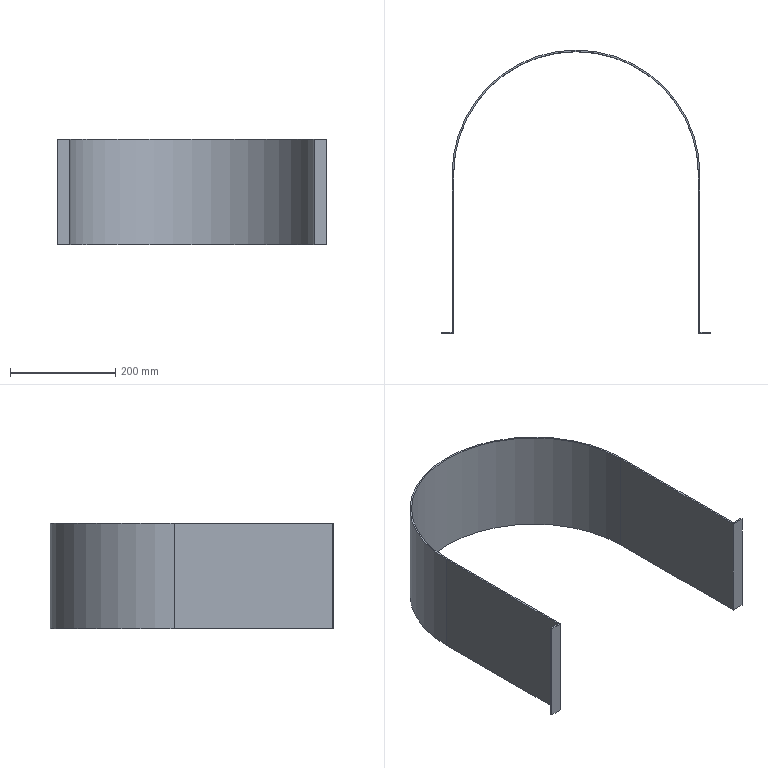Part | STEP file | Dust cover | 1 solid | 14 faces | box 510 x 538 x 200 mm | volume 827737 mm3 | plane 12 | cylinder 2 | commonest cylinder face diameters 464 x1 470 x1
STEP:
#1=CARTESIAN_POINT('',(0.,0.,0.));
#2=DIRECTION('',(0.,0.,1.));
#3=DIRECTION('',(1.,0.,0.));
#4=AXIS2_PLACEMENT_3D('',#1,#2,#3);
#5=CARTESIAN_POINT('',(-235.,-300.,-100.));
#6=VERTEX_POINT('',#5);
#7=CARTESIAN_POINT('',(-255.,-300.,-100.));
#8=VERTEX_POINT('',#7);
#9=CARTESIAN_POINT('',(-235.,-300.,-100.));
#10=DIRECTION('',(-1.,0.,0.));
#11=VECTOR('',#10,1.);
#12=LINE('',#9,#11);
#13=CARTESIAN_POINT('',(-235.,-300.,100.));
#14=DIRECTION('',(0.,-1.,0.));
#15=DIRECTION('',(1.,0.,0.));
#16=AXIS2_PLACEMENT_3D('',#13,#14,#15);
#17=PLANE('',#16);
#18=CARTESIAN_POINT('',(0.,-200.));
#19=DIRECTION('',(-1.,0.));
#20=VECTOR('',#19,1.);
#21=LINE('',#18,#20);
#22=(GEOMETRIC_REPRESENTATION_CONTEXT(2)PARAMETRIC_REPRESENTATION_CONTEXT()REPRESENTATION_CONTEXT('',''));
#23=DEFINITIONAL_REPRESENTATION('',(#21),#22);
#24=PCURVE('',#17,#23);
#25=CARTESIAN_POINT('',(0.,0.,-100.));
#26=DIRECTION('',(0.,0.,1.));
#27=DIRECTION('',(1.,0.,0.));
#28=AXIS2_PLACEMENT_3D('',#25,#26,#27);
#29=PLANE('',#28);
#30=CARTESIAN_POINT('',(-235.,-300.));
#31=DIRECTION('',(-1.,0.));
#32=VECTOR('',#31,1.);
#33=LINE('',#30,#32);
#34=(GEOMETRIC_REPRESENTATION_CONTEXT(2)PARAMETRIC_REPRESENTATION_CONTEXT()REPRESENTATION_CONTEXT('',''));
#35=DEFINITIONAL_REPRESENTATION('',(#33),#34);
#36=PCURVE('',#29,#35);
#37=SURFACE_CURVE('',#12,(#24,#36),.PCURVE_S1.);
#38=EDGE_CURVE('',#6,#8,#37,.T.);
#39=ORIENTED_EDGE('',*,*,#38,.T.);
#40=CARTESIAN_POINT('',(-255.,-300.,100.));
#41=VERTEX_POINT('',#40);
#42=CARTESIAN_POINT('',(-255.,-300.,100.));
#43=DIRECTION('',(0.,0.,-1.));
#44=VECTOR('',#43,1.);
#45=LINE('',#42,#44);
#46=CARTESIAN_POINT('',(-20.,0.));
#47=DIRECTION('',(0.,-1.));
#48=VECTOR('',#47,1.);
#49=LINE('',#46,#48);
#50=(GEOMETRIC_REPRESENTATION_CONTEXT(2)PARAMETRIC_REPRESENTATION_CONTEXT()REPRESENTATION_CONTEXT('',''));
#51=DEFINITIONAL_REPRESENTATION('',(#49),#50);
#52=PCURVE('',#17,#51);
#53=CARTESIAN_POINT('',(-255.,-303.,100.));
#54=DIRECTION('',(-1.,0.,0.));
#55=DIRECTION('',(0.,0.,1.));
#56=AXIS2_PLACEMENT_3D('',#53,#54,#55);
#57=PLANE('',#56);
#58=CARTESIAN_POINT('',(0.,3.));
#59=DIRECTION('',(-1.,0.));
#60=VECTOR('',#59,1.);
#61=LINE('',#58,#60);
#62=(GEOMETRIC_REPRESENTATION_CONTEXT(2)PARAMETRIC_REPRESENTATION_CONTEXT()REPRESENTATION_CONTEXT('',''));
#63=DEFINITIONAL_REPRESENTATION('',(#61),#62);
#64=PCURVE('',#57,#63);
#65=SURFACE_CURVE('',#45,(#52,#64),.PCURVE_S1.);
#66=EDGE_CURVE('',#41,#8,#65,.T.);
#67=ORIENTED_EDGE('',*,*,#66,.F.);
#68=CARTESIAN_POINT('',(-235.,-300.,100.));
#69=VERTEX_POINT('',#68);
#70=CARTESIAN_POINT('',(-235.,-300.,100.));
#71=DIRECTION('',(-1.,0.,0.));
#72=VECTOR('',#71,1.);
#73=LINE('',#70,#72);
#74=CARTESIAN_POINT('',(0.,0.));
#75=DIRECTION('',(-1.,0.));
#76=VECTOR('',#75,1.);
#77=LINE('',#74,#76);
#78=(GEOMETRIC_REPRESENTATION_CONTEXT(2)PARAMETRIC_REPRESENTATION_CONTEXT()REPRESENTATION_CONTEXT('',''));
#79=DEFINITIONAL_REPRESENTATION('',(#77),#78);
#80=PCURVE('',#17,#79);
#81=CARTESIAN_POINT('',(0.,0.,100.));
#82=DIRECTION('',(0.,0.,1.));
#83=DIRECTION('',(1.,0.,0.));
#84=AXIS2_PLACEMENT_3D('',#81,#82,#83);
#85=PLANE('',#84);
#86=CARTESIAN_POINT('',(-235.,-300.));
#87=DIRECTION('',(-1.,0.));
#88=VECTOR('',#87,1.);
#89=LINE('',#86,#88);
#90=(GEOMETRIC_REPRESENTATION_CONTEXT(2)PARAMETRIC_REPRESENTATION_CONTEXT()REPRESENTATION_CONTEXT('',''));
#91=DEFINITIONAL_REPRESENTATION('',(#89),#90);
#92=PCURVE('',#85,#91);
#93=SURFACE_CURVE('',#73,(#80,#92),.PCURVE_S1.);
#94=EDGE_CURVE('',#69,#41,#93,.T.);
#95=ORIENTED_EDGE('',*,*,#94,.F.);
#96=CARTESIAN_POINT('',(-235.,-300.,100.));
#97=DIRECTION('',(0.,0.,-1.));
#98=VECTOR('',#97,1.);
#99=LINE('',#96,#98);
#100=CARTESIAN_POINT('',(0.,0.));
#101=DIRECTION('',(0.,-1.));
#102=VECTOR('',#101,1.);
#103=LINE('',#100,#102);
#104=(GEOMETRIC_REPRESENTATION_CONTEXT(2)PARAMETRIC_REPRESENTATION_CONTEXT()REPRESENTATION_CONTEXT('',''));
#105=DEFINITIONAL_REPRESENTATION('',(#103),#104);
#106=PCURVE('',#17,#105);
#107=CARTESIAN_POINT('',(-235.,0.,100.));
#108=DIRECTION('',(1.,0.,0.));
#109=DIRECTION('',(0.,1.,0.));
#110=AXIS2_PLACEMENT_3D('',#107,#108,#109);
#111=PLANE('',#110);
#112=CARTESIAN_POINT('',(-300.,0.));
#113=DIRECTION('',(0.,-1.));
#114=VECTOR('',#113,1.);
#115=LINE('',#112,#114);
#116=(GEOMETRIC_REPRESENTATION_CONTEXT(2)PARAMETRIC_REPRESENTATION_CONTEXT()REPRESENTATION_CONTEXT('',''));
#117=DEFINITIONAL_REPRESENTATION('',(#115),#116);
#118=PCURVE('',#111,#117);
#119=SURFACE_CURVE('',#99,(#106,#118),.PCURVE_S1.);
#120=EDGE_CURVE('',#69,#6,#119,.T.);
#121=ORIENTED_EDGE('',*,*,#120,.T.);
#122=EDGE_LOOP('',(#39,#67,#95,#121));
#123=FACE_BOUND('',#122,.T.);
#124=ADVANCED_FACE('',(#123),#17,.F.);
#125=CARTESIAN_POINT('',(-255.,-303.,-100.));
#126=VERTEX_POINT('',#125);
#127=CARTESIAN_POINT('',(-255.,-303.,-100.));
#128=DIRECTION('',(0.,1.,0.));
#129=VECTOR('',#128,1.);
#130=LINE('',#127,#129);
#131=CARTESIAN_POINT('',(-200.,0.));
#132=DIRECTION('',(0.,1.));
#133=VECTOR('',#132,1.);
#134=LINE('',#131,#133);
#135=(GEOMETRIC_REPRESENTATION_CONTEXT(2)PARAMETRIC_REPRESENTATION_CONTEXT()REPRESENTATION_CONTEXT('',''));
#136=DEFINITIONAL_REPRESENTATION('',(#134),#135);
#137=PCURVE('',#57,#136);
#138=CARTESIAN_POINT('',(-255.,-303.));
#139=DIRECTION('',(0.,1.));
#140=VECTOR('',#139,1.);
#141=LINE('',#138,#140);
#142=(GEOMETRIC_REPRESENTATION_CONTEXT(2)PARAMETRIC_REPRESENTATION_CONTEXT()REPRESENTATION_CONTEXT('',''));
#143=DEFINITIONAL_REPRESENTATION('',(#141),#142);
#144=PCURVE('',#29,#143);
#145=SURFACE_CURVE('',#130,(#137,#144),.PCURVE_S1.);
#146=EDGE_CURVE('',#126,#8,#145,.T.);
#147=ORIENTED_EDGE('',*,*,#146,.F.);
#148=CARTESIAN_POINT('',(-255.,-303.,100.));
#149=VERTEX_POINT('',#148);
#150=CARTESIAN_POINT('',(-255.,-303.,100.));
#151=DIRECTION('',(0.,0.,-1.));
#152=VECTOR('',#151,1.);
#153=LINE('',#150,#152);
#154=CARTESIAN_POINT('',(0.,0.));
#155=DIRECTION('',(-1.,0.));
#156=VECTOR('',#155,1.);
#157=LINE('',#154,#156);
#158=(GEOMETRIC_REPRESENTATION_CONTEXT(2)PARAMETRIC_REPRESENTATION_CONTEXT()REPRESENTATION_CONTEXT('',''));
#159=DEFINITIONAL_REPRESENTATION('',(#157),#158);
#160=PCURVE('',#57,#159);
#161=CARTESIAN_POINT('',(-235.,-303.,100.));
#162=DIRECTION('',(0.,-1.,0.));
#163=DIRECTION('',(1.,0.,0.));
#164=AXIS2_PLACEMENT_3D('',#161,#162,#163);
#165=PLANE('',#164);
#166=CARTESIAN_POINT('',(-20.,0.));
#167=DIRECTION('',(0.,-1.));
#168=VECTOR('',#167,1.);
#169=LINE('',#166,#168);
#170=(GEOMETRIC_REPRESENTATION_CONTEXT(2)PARAMETRIC_REPRESENTATION_CONTEXT()REPRESENTATION_CONTEXT('',''));
#171=DEFINITIONAL_REPRESENTATION('',(#169),#170);
#172=PCURVE('',#165,#171);
#173=SURFACE_CURVE('',#153,(#160,#172),.PCURVE_S1.);
#174=EDGE_CURVE('',#149,#126,#173,.T.);
#175=ORIENTED_EDGE('',*,*,#174,.F.);
#176=CARTESIAN_POINT('',(-255.,-303.,100.));
#177=DIRECTION('',(0.,1.,0.));
#178=VECTOR('',#177,1.);
#179=LINE('',#176,#178);
#180=CARTESIAN_POINT('',(0.,0.));
#181=DIRECTION('',(0.,1.));
#182=VECTOR('',#181,1.);
#183=LINE('',#180,#182);
#184=(GEOMETRIC_REPRESENTATION_CONTEXT(2)PARAMETRIC_REPRESENTATION_CONTEXT()REPRESENTATION_CONTEXT('',''));
#185=DEFINITIONAL_REPRESENTATION('',(#183),#184);
#186=PCURVE('',#57,#185);
#187=CARTESIAN_POINT('',(-255.,-303.));
#188=DIRECTION('',(0.,1.));
#189=VECTOR('',#188,1.);
#190=LINE('',#187,#189);
#191=(GEOMETRIC_REPRESENTATION_CONTEXT(2)PARAMETRIC_REPRESENTATION_CONTEXT()REPRESENTATION_CONTEXT('',''));
#192=DEFINITIONAL_REPRESENTATION('',(#190),#191);
#193=PCURVE('',#85,#192);
#194=SURFACE_CURVE('',#179,(#186,#193),.PCURVE_S1.);
#195=EDGE_CURVE('',#149,#41,#194,.T.);
#196=ORIENTED_EDGE('',*,*,#195,.T.);
#197=ORIENTED_EDGE('',*,*,#66,.T.);
#198=EDGE_LOOP('',(#147,#175,#196,#197));
#199=FACE_BOUND('',#198,.T.);
#200=ADVANCED_FACE('',(#199),#57,.T.);
#201=CARTESIAN_POINT('',(-232.,-303.,-100.));
#202=VERTEX_POINT('',#201);
#203=CARTESIAN_POINT('',(-235.,-303.,-100.));
#204=DIRECTION('',(-1.,0.,0.));
#205=VECTOR('',#204,1.);
#206=LINE('',#203,#205);
#207=CARTESIAN_POINT('',(0.,-200.));
#208=DIRECTION('',(-1.,0.));
#209=VECTOR('',#208,1.);
#210=LINE('',#207,#209);
#211=(GEOMETRIC_REPRESENTATION_CONTEXT(2)PARAMETRIC_REPRESENTATION_CONTEXT()REPRESENTATION_CONTEXT('',''));
#212=DEFINITIONAL_REPRESENTATION('',(#210),#211);
#213=PCURVE('',#165,#212);
#214=CARTESIAN_POINT('',(-235.,-303.));
#215=DIRECTION('',(-1.,0.));
#216=VECTOR('',#215,1.);
#217=LINE('',#214,#216);
#218=(GEOMETRIC_REPRESENTATION_CONTEXT(2)PARAMETRIC_REPRESENTATION_CONTEXT()REPRESENTATION_CONTEXT('',''));
#219=DEFINITIONAL_REPRESENTATION('',(#217),#218);
#220=PCURVE('',#29,#219);
#221=SURFACE_CURVE('',#206,(#213,#220),.PCURVE_S1.);
#222=EDGE_CURVE('',#202,#126,#221,.T.);
#223=ORIENTED_EDGE('',*,*,#222,.F.);
#224=CARTESIAN_POINT('',(-232.,-303.,100.));
#225=VERTEX_POINT('',#224);
#226=CARTESIAN_POINT('',(-232.,-303.,100.));
#227=DIRECTION('',(0.,0.,-1.));
#228=VECTOR('',#227,1.);
#229=LINE('',#226,#228);
#230=CARTESIAN_POINT('',(3.,0.));
#231=DIRECTION('',(0.,-1.));
#232=VECTOR('',#231,1.);
#233=LINE('',#230,#232);
#234=(GEOMETRIC_REPRESENTATION_CONTEXT(2)PARAMETRIC_REPRESENTATION_CONTEXT()REPRESENTATION_CONTEXT('',''));
#235=DEFINITIONAL_REPRESENTATION('',(#233),#234);
#236=PCURVE('',#165,#235);
#237=CARTESIAN_POINT('',(-232.,0.,100.));
#238=DIRECTION('',(1.,0.,0.));
#239=DIRECTION('',(0.,1.,0.));
#240=AXIS2_PLACEMENT_3D('',#237,#238,#239);
#241=PLANE('',#240);
#242=CARTESIAN_POINT('',(-303.,0.));
#243=DIRECTION('',(0.,-1.));
#244=VECTOR('',#243,1.);
#245=LINE('',#242,#244);
#246=(GEOMETRIC_REPRESENTATION_CONTEXT(2)PARAMETRIC_REPRESENTATION_CONTEXT()REPRESENTATION_CONTEXT('',''));
#247=DEFINITIONAL_REPRESENTATION('',(#245),#246);
#248=PCURVE('',#241,#247);
#249=SURFACE_CURVE('',#229,(#236,#248),.PCURVE_S1.);
#250=EDGE_CURVE('',#225,#202,#249,.T.);
#251=ORIENTED_EDGE('',*,*,#250,.F.);
#252=CARTESIAN_POINT('',(-235.,-303.,100.));
#253=DIRECTION('',(-1.,0.,0.));
#254=VECTOR('',#253,1.);
#255=LINE('',#252,#254);
#256=CARTESIAN_POINT('',(0.,0.));
#257=DIRECTION('',(-1.,0.));
#258=VECTOR('',#257,1.);
#259=LINE('',#256,#258);
#260=(GEOMETRIC_REPRESENTATION_CONTEXT(2)PARAMETRIC_REPRESENTATION_CONTEXT()REPRESENTATION_CONTEXT('',''));
#261=DEFINITIONAL_REPRESENTATION('',(#259),#260);
#262=PCURVE('',#165,#261);
#263=CARTESIAN_POINT('',(-235.,-303.));
#264=DIRECTION('',(-1.,0.));
#265=VECTOR('',#264,1.);
#266=LINE('',#263,#265);
#267=(GEOMETRIC_REPRESENTATION_CONTEXT(2)PARAMETRIC_REPRESENTATION_CONTEXT()REPRESENTATION_CONTEXT('',''));
#268=DEFINITIONAL_REPRESENTATION('',(#266),#267);
#269=PCURVE('',#85,#268);
#270=SURFACE_CURVE('',#255,(#262,#269),.PCURVE_S1.);
#271=EDGE_CURVE('',#225,#149,#270,.T.);
#272=ORIENTED_EDGE('',*,*,#271,.T.);
#273=ORIENTED_EDGE('',*,*,#174,.T.);
#274=EDGE_LOOP('',(#223,#251,#272,#273));
#275=FACE_BOUND('',#274,.T.);
#276=ADVANCED_FACE('',(#275),#165,.T.);
#277=CARTESIAN_POINT('',(-232.,0.,-100.));
#278=VERTEX_POINT('',#277);
#279=CARTESIAN_POINT('',(-232.,0.,-100.));
#280=DIRECTION('',(0.,-1.,0.));
#281=VECTOR('',#280,1.);
#282=LINE('',#279,#281);
#283=CARTESIAN_POINT('',(0.,-200.));
#284=DIRECTION('',(-1.,0.));
#285=VECTOR('',#284,1.);
#286=LINE('',#283,#285);
#287=(GEOMETRIC_REPRESENTATION_CONTEXT(2)PARAMETRIC_REPRESENTATION_CONTEXT()REPRESENTATION_CONTEXT('',''));
#288=DEFINITIONAL_REPRESENTATION('',(#286),#287);
#289=PCURVE('',#241,#288);
#290=CARTESIAN_POINT('',(-232.,0.));
#291=DIRECTION('',(0.,-1.));
#292=VECTOR('',#291,1.);
#293=LINE('',#290,#292);
#294=(GEOMETRIC_REPRESENTATION_CONTEXT(2)PARAMETRIC_REPRESENTATION_CONTEXT()REPRESENTATION_CONTEXT('',''));
#295=DEFINITIONAL_REPRESENTATION('',(#293),#294);
#296=PCURVE('',#29,#295);
#297=SURFACE_CURVE('',#282,(#289,#296),.PCURVE_S1.);
#298=EDGE_CURVE('',#278,#202,#297,.T.);
#299=ORIENTED_EDGE('',*,*,#298,.F.);
#300=CARTESIAN_POINT('',(-232.,0.,100.));
#301=VERTEX_POINT('',#300);
#302=CARTESIAN_POINT('',(-232.,0.,100.));
#303=DIRECTION('',(0.,0.,-1.));
#304=VECTOR('',#303,1.);
#305=LINE('',#302,#304);
#306=CARTESIAN_POINT('',(0.,0.));
#307=DIRECTION('',(0.,-1.));
#308=VECTOR('',#307,1.);
#309=LINE('',#306,#308);
#310=(GEOMETRIC_REPRESENTATION_CONTEXT(2)PARAMETRIC_REPRESENTATION_CONTEXT()REPRESENTATION_CONTEXT('',''));
#311=DEFINITIONAL_REPRESENTATION('',(#309),#310);
#312=PCURVE('',#241,#311);
#313=CARTESIAN_POINT('',(0.,0.,100.));
#314=DIRECTION('',(0.,0.,-1.));
#315=DIRECTION('',(-1.,0.,0.));
#316=AXIS2_PLACEMENT_3D('',#313,#314,#315);
#317=CYLINDRICAL_SURFACE('',#316,232.);
#318=CARTESIAN_POINT('',(0.,0.));
#319=DIRECTION('',(0.,1.));
#320=VECTOR('',#319,1.);
#321=LINE('',#318,#320);
#322=(GEOMETRIC_REPRESENTATION_CONTEXT(2)PARAMETRIC_REPRESENTATION_CONTEXT()REPRESENTATION_CONTEXT('',''));
#323=DEFINITIONAL_REPRESENTATION('',(#321),#322);
#324=PCURVE('',#317,#323);
#325=SURFACE_CURVE('',#305,(#312,#324),.PCURVE_S1.);
#326=EDGE_CURVE('',#301,#278,#325,.T.);
#327=ORIENTED_EDGE('',*,*,#326,.F.);
#328=CARTESIAN_POINT('',(-232.,0.,100.));
#329=DIRECTION('',(0.,-1.,0.));
#330=VECTOR('',#329,1.);
#331=LINE('',#328,#330);
#332=CARTESIAN_POINT('',(0.,0.));
#333=DIRECTION('',(-1.,0.));
#334=VECTOR('',#333,1.);
#335=LINE('',#332,#334);
#336=(GEOMETRIC_REPRESENTATION_CONTEXT(2)PARAMETRIC_REPRESENTATION_CONTEXT()REPRESENTATION_CONTEXT('',''));
#337=DEFINITIONAL_REPRESENTATION('',(#335),#336);
#338=PCURVE('',#241,#337);
#339=CARTESIAN_POINT('',(-232.,0.));
#340=DIRECTION('',(0.,-1.));
#341=VECTOR('',#340,1.);
#342=LINE('',#339,#341);
#343=(GEOMETRIC_REPRESENTATION_CONTEXT(2)PARAMETRIC_REPRESENTATION_CONTEXT()REPRESENTATION_CONTEXT('',''));
#344=DEFINITIONAL_REPRESENTATION('',(#342),#343);
#345=PCURVE('',#85,#344);
#346=SURFACE_CURVE('',#331,(#338,#345),.PCURVE_S1.);
#347=EDGE_CURVE('',#301,#225,#346,.T.);
#348=ORIENTED_EDGE('',*,*,#347,.T.);
#349=ORIENTED_EDGE('',*,*,#250,.T.);
#350=EDGE_LOOP('',(#299,#327,#348,#349));
#351=FACE_BOUND('',#350,.T.);
#352=ADVANCED_FACE('',(#351),#241,.T.);
#353=ORIENTED_EDGE('',*,*,#326,.F.);
#354=CARTESIAN_POINT('',(232.,0.,100.));
#355=VERTEX_POINT('',#354);
#356=CARTESIAN_POINT('',(0.,0.,100.));
#357=DIRECTION('',(0.,0.,1.));
#358=DIRECTION('',(1.,0.,0.));
#359=AXIS2_PLACEMENT_3D('',#356,#357,#358);
#360=CIRCLE('',#359,232.);
#361=CARTESIAN_POINT('',(3.142,0.));
#362=DIRECTION('',(-1.,0.));
#363=VECTOR('',#362,1.);
#364=LINE('',#361,#363);
#365=(GEOMETRIC_REPRESENTATION_CONTEXT(2)PARAMETRIC_REPRESENTATION_CONTEXT()REPRESENTATION_CONTEXT('',''));
#366=DEFINITIONAL_REPRESENTATION('',(#364),#365);
#367=PCURVE('',#317,#366);
#368=CARTESIAN_POINT('',(0.,0.));
#369=DIRECTION('',(1.,0.));
#370=AXIS2_PLACEMENT_2D('',#368,#369);
#371=CIRCLE('',#370,232.);
#372=(GEOMETRIC_REPRESENTATION_CONTEXT(2)PARAMETRIC_REPRESENTATION_CONTEXT()REPRESENTATION_CONTEXT('',''));
#373=DEFINITIONAL_REPRESENTATION('',(#371),#372);
#374=PCURVE('',#85,#373);
#375=SURFACE_CURVE('',#360,(#367,#374),.PCURVE_S1.);
#376=EDGE_CURVE('',#355,#301,#375,.T.);
#377=ORIENTED_EDGE('',*,*,#376,.F.);
#378=CARTESIAN_POINT('',(232.,0.,-100.));
#379=VERTEX_POINT('',#378);
#380=CARTESIAN_POINT('',(232.,0.,100.));
#381=DIRECTION('',(0.,0.,-1.));
#382=VECTOR('',#381,1.);
#383=LINE('',#380,#382);
#384=CARTESIAN_POINT('',(3.142,0.));
#385=DIRECTION('',(0.,1.));
#386=VECTOR('',#385,1.);
#387=LINE('',#384,#386);
#388=(GEOMETRIC_REPRESENTATION_CONTEXT(2)PARAMETRIC_REPRESENTATION_CONTEXT()REPRESENTATION_CONTEXT('',''));
#389=DEFINITIONAL_REPRESENTATION('',(#387),#388);
#390=PCURVE('',#317,#389);
#391=CARTESIAN_POINT('',(232.,0.,100.));
#392=DIRECTION('',(-1.,0.,0.));
#393=DIRECTION('',(0.,-1.,0.));
#394=AXIS2_PLACEMENT_3D('',#391,#392,#393);
#395=PLANE('',#394);
#396=CARTESIAN_POINT('',(0.,0.));
#397=DIRECTION('',(0.,-1.));
#398=VECTOR('',#397,1.);
#399=LINE('',#396,#398);
#400=(GEOMETRIC_REPRESENTATION_CONTEXT(2)PARAMETRIC_REPRESENTATION_CONTEXT()REPRESENTATION_CONTEXT('',''));
#401=DEFINITIONAL_REPRESENTATION('',(#399),#400);
#402=PCURVE('',#395,#401);
#403=SURFACE_CURVE('',#383,(#390,#402),.PCURVE_S1.);
#404=EDGE_CURVE('',#355,#379,#403,.T.);
#405=ORIENTED_EDGE('',*,*,#404,.T.);
#406=CARTESIAN_POINT('',(0.,0.,-100.));
#407=DIRECTION('',(0.,0.,1.));
#408=DIRECTION('',(1.,0.,0.));
#409=AXIS2_PLACEMENT_3D('',#406,#407,#408);
#410=CIRCLE('',#409,232.);
#411=CARTESIAN_POINT('',(3.142,200.));
#412=DIRECTION('',(-1.,0.));
#413=VECTOR('',#412,1.);
#414=LINE('',#411,#413);
#415=(GEOMETRIC_REPRESENTATION_CONTEXT(2)PARAMETRIC_REPRESENTATION_CONTEXT()REPRESENTATION_CONTEXT('',''));
#416=DEFINITIONAL_REPRESENTATION('',(#414),#415);
#417=PCURVE('',#317,#416);
#418=CARTESIAN_POINT('',(0.,0.));
#419=DIRECTION('',(1.,0.));
#420=AXIS2_PLACEMENT_2D('',#418,#419);
#421=CIRCLE('',#420,232.);
#422=(GEOMETRIC_REPRESENTATION_CONTEXT(2)PARAMETRIC_REPRESENTATION_CONTEXT()REPRESENTATION_CONTEXT('',''));
#423=DEFINITIONAL_REPRESENTATION('',(#421),#422);
#424=PCURVE('',#29,#423);
#425=SURFACE_CURVE('',#410,(#417,#424),.PCURVE_S1.);
#426=EDGE_CURVE('',#379,#278,#425,.T.);
#427=ORIENTED_EDGE('',*,*,#426,.T.);
#428=EDGE_LOOP('',(#353,#377,#405,#427));
#429=FACE_BOUND('',#428,.F.);
#430=ADVANCED_FACE('',(#429),#317,.F.);
#431=CARTESIAN_POINT('',(232.,-303.,-100.));
#432=VERTEX_POINT('',#431);
#433=CARTESIAN_POINT('',(232.,0.,-100.));
#434=DIRECTION('',(0.,1.,0.));
#435=VECTOR('',#434,1.);
#436=LINE('',#433,#435);
#437=CARTESIAN_POINT('',(0.,-200.));
#438=DIRECTION('',(-1.,0.));
#439=VECTOR('',#438,1.);
#440=LINE('',#437,#439);
#441=(GEOMETRIC_REPRESENTATION_CONTEXT(2)PARAMETRIC_REPRESENTATION_CONTEXT()REPRESENTATION_CONTEXT('',''));
#442=DEFINITIONAL_REPRESENTATION('',(#440),#441);
#443=PCURVE('',#395,#442);
#444=CARTESIAN_POINT('',(232.,0.));
#445=DIRECTION('',(0.,1.));
#446=VECTOR('',#445,1.);
#447=LINE('',#444,#446);
#448=(GEOMETRIC_REPRESENTATION_CONTEXT(2)PARAMETRIC_REPRESENTATION_CONTEXT()REPRESENTATION_CONTEXT('',''));
#449=DEFINITIONAL_REPRESENTATION('',(#447),#448);
#450=PCURVE('',#29,#449);
#451=SURFACE_CURVE('',#436,(#443,#450),.PCURVE_S1.);
#452=EDGE_CURVE('',#432,#379,#451,.T.);
#453=ORIENTED_EDGE('',*,*,#452,.F.);
#454=CARTESIAN_POINT('',(232.,-303.,100.));
#455=VERTEX_POINT('',#454);
#456=CARTESIAN_POINT('',(232.,-303.,100.));
#457=DIRECTION('',(0.,0.,-1.));
#458=VECTOR('',#457,1.);
#459=LINE('',#456,#458);
#460=CARTESIAN_POINT('',(303.,0.));
#461=DIRECTION('',(0.,-1.));
#462=VECTOR('',#461,1.);
#463=LINE('',#460,#462);
#464=(GEOMETRIC_REPRESENTATION_CONTEXT(2)PARAMETRIC_REPRESENTATION_CONTEXT()REPRESENTATION_CONTEXT('',''));
#465=DEFINITIONAL_REPRESENTATION('',(#463),#464);
#466=PCURVE('',#395,#465);
#467=CARTESIAN_POINT('',(235.,-303.,100.));
#468=DIRECTION('',(0.,-1.,0.));
#469=DIRECTION('',(1.,0.,0.));
#470=AXIS2_PLACEMENT_3D('',#467,#468,#469);
#471=PLANE('',#470);
#472=CARTESIAN_POINT('',(-3.,0.));
#473=DIRECTION('',(0.,-1.));
#474=VECTOR('',#473,1.);
#475=LINE('',#472,#474);
#476=(GEOMETRIC_REPRESENTATION_CONTEXT(2)PARAMETRIC_REPRESENTATION_CONTEXT()REPRESENTATION_CONTEXT('',''));
#477=DEFINITIONAL_REPRESENTATION('',(#475),#476);
#478=PCURVE('',#471,#477);
#479=SURFACE_CURVE('',#459,(#466,#478),.PCURVE_S1.);
#480=EDGE_CURVE('',#455,#432,#479,.T.);
#481=ORIENTED_EDGE('',*,*,#480,.F.);
#482=CARTESIAN_POINT('',(232.,0.,100.));
#483=DIRECTION('',(0.,1.,0.));
#484=VECTOR('',#483,1.);
#485=LINE('',#482,#484);
#486=CARTESIAN_POINT('',(0.,0.));
#487=DIRECTION('',(-1.,0.));
#488=VECTOR('',#487,1.);
#489=LINE('',#486,#488);
#490=(GEOMETRIC_REPRESENTATION_CONTEXT(2)PARAMETRIC_REPRESENTATION_CONTEXT()REPRESENTATION_CONTEXT('',''));
#491=DEFINITIONAL_REPRESENTATION('',(#489),#490);
#492=PCURVE('',#395,#491);
#493=CARTESIAN_POINT('',(232.,0.));
#494=DIRECTION('',(0.,1.));
#495=VECTOR('',#494,1.);
#496=LINE('',#493,#495);
#497=(GEOMETRIC_REPRESENTATION_CONTEXT(2)PARAMETRIC_REPRESENTATION_CONTEXT()REPRESENTATION_CONTEXT('',''));
#498=DEFINITIONAL_REPRESENTATION('',(#496),#497);
#499=PCURVE('',#85,#498);
#500=SURFACE_CURVE('',#485,(#492,#499),.PCURVE_S1.);
#501=EDGE_CURVE('',#455,#355,#500,.T.);
#502=ORIENTED_EDGE('',*,*,#501,.T.);
#503=ORIENTED_EDGE('',*,*,#404,.T.);
#504=EDGE_LOOP('',(#453,#481,#502,#503));
#505=FACE_BOUND('',#504,.T.);
#506=ADVANCED_FACE('',(#505),#395,.T.);
#507=CARTESIAN_POINT('',(255.,-303.,-100.));
#508=VERTEX_POINT('',#507);
#509=CARTESIAN_POINT('',(235.,-303.,-100.));
#510=DIRECTION('',(-1.,0.,0.));
#511=VECTOR('',#510,1.);
#512=LINE('',#509,#511);
#513=CARTESIAN_POINT('',(0.,-200.));
#514=DIRECTION('',(-1.,0.));
#515=VECTOR('',#514,1.);
#516=LINE('',#513,#515);
#517=(GEOMETRIC_REPRESENTATION_CONTEXT(2)PARAMETRIC_REPRESENTATION_CONTEXT()REPRESENTATION_CONTEXT('',''));
#518=DEFINITIONAL_REPRESENTATION('',(#516),#517);
#519=PCURVE('',#471,#518);
#520=CARTESIAN_POINT('',(235.,-303.));
#521=DIRECTION('',(-1.,0.));
#522=VECTOR('',#521,1.);
#523=LINE('',#520,#522);
#524=(GEOMETRIC_REPRESENTATION_CONTEXT(2)PARAMETRIC_REPRESENTATION_CONTEXT()REPRESENTATION_CONTEXT('',''));
#525=DEFINITIONAL_REPRESENTATION('',(#523),#524);
#526=PCURVE('',#29,#525);
#527=SURFACE_CURVE('',#512,(#519,#526),.PCURVE_S1.);
#528=EDGE_CURVE('',#508,#432,#527,.T.);
#529=ORIENTED_EDGE('',*,*,#528,.F.);
#530=CARTESIAN_POINT('',(255.,-303.,100.));
#531=VERTEX_POINT('',#530);
#532=CARTESIAN_POINT('',(255.,-303.,100.));
#533=DIRECTION('',(0.,0.,-1.));
#534=VECTOR('',#533,1.);
#535=LINE('',#532,#534);
#536=CARTESIAN_POINT('',(20.,0.));
#537=DIRECTION('',(0.,-1.));
#538=VECTOR('',#537,1.);
#539=LINE('',#536,#538);
#540=(GEOMETRIC_REPRESENTATION_CONTEXT(2)PARAMETRIC_REPRESENTATION_CONTEXT()REPRESENTATION_CONTEXT('',''));
#541=DEFINITIONAL_REPRESENTATION('',(#539),#540);
#542=PCURVE('',#471,#541);
#543=CARTESIAN_POINT('',(255.,-300.,100.));
#544=DIRECTION('',(1.,0.,0.));
#545=DIRECTION('',(0.,0.,-1.));
#546=AXIS2_PLACEMENT_3D('',#543,#544,#545);
#547=PLANE('',#546);
#548=CARTESIAN_POINT('',(0.,-3.));
#549=DIRECTION('',(1.,0.));
#550=VECTOR('',#549,1.);
#551=LINE('',#548,#550);
#552=(GEOMETRIC_REPRESENTATION_CONTEXT(2)PARAMETRIC_REPRESENTATION_CONTEXT()REPRESENTATION_CONTEXT('',''));
#553=DEFINITIONAL_REPRESENTATION('',(#551),#552);
#554=PCURVE('',#547,#553);
#555=SURFACE_CURVE('',#535,(#542,#554),.PCURVE_S1.);
#556=EDGE_CURVE('',#531,#508,#555,.T.);
#557=ORIENTED_EDGE('',*,*,#556,.F.);
#558=CARTESIAN_POINT('',(235.,-303.,100.));
#559=DIRECTION('',(-1.,0.,0.));
#560=VECTOR('',#559,1.);
#561=LINE('',#558,#560);
#562=CARTESIAN_POINT('',(0.,0.));
#563=DIRECTION('',(-1.,0.));
#564=VECTOR('',#563,1.);
#565=LINE('',#562,#564);
#566=(GEOMETRIC_REPRESENTATION_CONTEXT(2)PARAMETRIC_REPRESENTATION_CONTEXT()REPRESENTATION_CONTEXT('',''));
#567=DEFINITIONAL_REPRESENTATION('',(#565),#566);
#568=PCURVE('',#471,#567);
#569=CARTESIAN_POINT('',(235.,-303.));
#570=DIRECTION('',(-1.,0.));
#571=VECTOR('',#570,1.);
#572=LINE('',#569,#571);
#573=(GEOMETRIC_REPRESENTATION_CONTEXT(2)PARAMETRIC_REPRESENTATION_CONTEXT()REPRESENTATION_CONTEXT('',''));
#574=DEFINITIONAL_REPRESENTATION('',(#572),#573);
#575=PCURVE('',#85,#574);
#576=SURFACE_CURVE('',#561,(#568,#575),.PCURVE_S1.);
#577=EDGE_CURVE('',#531,#455,#576,.T.);
#578=ORIENTED_EDGE('',*,*,#577,.T.);
#579=ORIENTED_EDGE('',*,*,#480,.T.);
#580=EDGE_LOOP('',(#529,#557,#578,#579));
#581=FACE_BOUND('',#580,.T.);
#582=ADVANCED_FACE('',(#581),#471,.T.);
#583=CARTESIAN_POINT('',(255.,-300.,-100.));
#584=VERTEX_POINT('',#583);
#585=CARTESIAN_POINT('',(255.,-300.,-100.));
#586=DIRECTION('',(0.,-1.,0.));
#587=VECTOR('',#586,1.);
#588=LINE('',#585,#587);
#589=CARTESIAN_POINT('',(200.,0.));
#590=DIRECTION('',(0.,-1.));
#591=VECTOR('',#590,1.);
#592=LINE('',#589,#591);
#593=(GEOMETRIC_REPRESENTATION_CONTEXT(2)PARAMETRIC_REPRESENTATION_CONTEXT()REPRESENTATION_CONTEXT('',''));
#594=DEFINITIONAL_REPRESENTATION('',(#592),#593);
#595=PCURVE('',#547,#594);
#596=CARTESIAN_POINT('',(255.,-300.));
#597=DIRECTION('',(0.,-1.));
#598=VECTOR('',#597,1.);
#599=LINE('',#596,#598);
#600=(GEOMETRIC_REPRESENTATION_CONTEXT(2)PARAMETRIC_REPRESENTATION_CONTEXT()REPRESENTATION_CONTEXT('',''));
#601=DEFINITIONAL_REPRESENTATION('',(#599),#600);
#602=PCURVE('',#29,#601);
#603=SURFACE_CURVE('',#588,(#595,#602),.PCURVE_S1.);
#604=EDGE_CURVE('',#584,#508,#603,.T.);
#605=ORIENTED_EDGE('',*,*,#604,.F.);
#606=CARTESIAN_POINT('',(255.,-300.,100.));
#607=VERTEX_POINT('',#606);
#608=CARTESIAN_POINT('',(255.,-300.,100.));
#609=DIRECTION('',(0.,0.,-1.));
#610=VECTOR('',#609,1.);
#611=LINE('',#608,#610);
#612=CARTESIAN_POINT('',(0.,0.));
#613=DIRECTION('',(1.,0.));
#614=VECTOR('',#613,1.);
#615=LINE('',#612,#614);
#616=(GEOMETRIC_REPRESENTATION_CONTEXT(2)PARAMETRIC_REPRESENTATION_CONTEXT()REPRESENTATION_CONTEXT('',''));
#617=DEFINITIONAL_REPRESENTATION('',(#615),#616);
#618=PCURVE('',#547,#617);
#619=CARTESIAN_POINT('',(235.,-300.,100.));
#620=DIRECTION('',(0.,-1.,0.));
#621=DIRECTION('',(1.,0.,0.));
#622=AXIS2_PLACEMENT_3D('',#619,#620,#621);
#623=PLANE('',#622);
#624=CARTESIAN_POINT('',(20.,0.));
#625=DIRECTION('',(0.,-1.));
#626=VECTOR('',#625,1.);
#627=LINE('',#624,#626);
#628=(GEOMETRIC_REPRESENTATION_CONTEXT(2)PARAMETRIC_REPRESENTATION_CONTEXT()REPRESENTATION_CONTEXT('',''));
#629=DEFINITIONAL_REPRESENTATION('',(#627),#628);
#630=PCURVE('',#623,#629);
#631=SURFACE_CURVE('',#611,(#618,#630),.PCURVE_S1.);
#632=EDGE_CURVE('',#607,#584,#631,.T.);
#633=ORIENTED_EDGE('',*,*,#632,.F.);
#634=CARTESIAN_POINT('',(255.,-300.,100.));
#635=DIRECTION('',(0.,-1.,0.));
#636=VECTOR('',#635,1.);
#637=LINE('',#634,#636);
#638=CARTESIAN_POINT('',(0.,0.));
#639=DIRECTION('',(0.,-1.));
#640=VECTOR('',#639,1.);
#641=LINE('',#638,#640);
#642=(GEOMETRIC_REPRESENTATION_CONTEXT(2)PARAMETRIC_REPRESENTATION_CONTEXT()REPRESENTATION_CONTEXT('',''));
#643=DEFINITIONAL_REPRESENTATION('',(#641),#642);
#644=PCURVE('',#547,#643);
#645=CARTESIAN_POINT('',(255.,-300.));
#646=DIRECTION('',(0.,-1.));
#647=VECTOR('',#646,1.);
#648=LINE('',#645,#647);
#649=(GEOMETRIC_REPRESENTATION_CONTEXT(2)PARAMETRIC_REPRESENTATION_CONTEXT()REPRESENTATION_CONTEXT('',''));
#650=DEFINITIONAL_REPRESENTATION('',(#648),#649);
#651=PCURVE('',#85,#650);
#652=SURFACE_CURVE('',#637,(#644,#651),.PCURVE_S1.);
#653=EDGE_CURVE('',#607,#531,#652,.T.);
#654=ORIENTED_EDGE('',*,*,#653,.T.);
#655=ORIENTED_EDGE('',*,*,#556,.T.);
#656=EDGE_LOOP('',(#605,#633,#654,#655));
#657=FACE_BOUND('',#656,.T.);
#658=ADVANCED_FACE('',(#657),#547,.T.);
#659=CARTESIAN_POINT('',(235.,-300.,-100.));
#660=VERTEX_POINT('',#659);
#661=CARTESIAN_POINT('',(235.,-300.,-100.));
#662=DIRECTION('',(-1.,0.,0.));
#663=VECTOR('',#662,1.);
#664=LINE('',#661,#663);
#665=CARTESIAN_POINT('',(0.,-200.));
#666=DIRECTION('',(-1.,0.));
#667=VECTOR('',#666,1.);
#668=LINE('',#665,#667);
#669=(GEOMETRIC_REPRESENTATION_CONTEXT(2)PARAMETRIC_REPRESENTATION_CONTEXT()REPRESENTATION_CONTEXT('',''));
#670=DEFINITIONAL_REPRESENTATION('',(#668),#669);
#671=PCURVE('',#623,#670);
#672=CARTESIAN_POINT('',(235.,-300.));
#673=DIRECTION('',(-1.,0.));
#674=VECTOR('',#673,1.);
#675=LINE('',#672,#674);
#676=(GEOMETRIC_REPRESENTATION_CONTEXT(2)PARAMETRIC_REPRESENTATION_CONTEXT()REPRESENTATION_CONTEXT('',''));
#677=DEFINITIONAL_REPRESENTATION('',(#675),#676);
#678=PCURVE('',#29,#677);
#679=SURFACE_CURVE('',#664,(#671,#678),.PCURVE_S1.);
#680=EDGE_CURVE('',#584,#660,#679,.T.);
#681=ORIENTED_EDGE('',*,*,#680,.T.);
#682=CARTESIAN_POINT('',(235.,-300.,100.));
#683=VERTEX_POINT('',#682);
#684=CARTESIAN_POINT('',(235.,-300.,100.));
#685=DIRECTION('',(0.,0.,-1.));
#686=VECTOR('',#685,1.);
#687=LINE('',#684,#686);
#688=CARTESIAN_POINT('',(0.,0.));
#689=DIRECTION('',(0.,-1.));
#690=VECTOR('',#689,1.);
#691=LINE('',#688,#690);
#692=(GEOMETRIC_REPRESENTATION_CONTEXT(2)PARAMETRIC_REPRESENTATION_CONTEXT()REPRESENTATION_CONTEXT('',''));
#693=DEFINITIONAL_REPRESENTATION('',(#691),#692);
#694=PCURVE('',#623,#693);
#695=CARTESIAN_POINT('',(235.,0.,100.));
#696=DIRECTION('',(-1.,0.,0.));
#697=DIRECTION('',(0.,-1.,0.));
#698=AXIS2_PLACEMENT_3D('',#695,#696,#697);
#699=PLANE('',#698);
#700=CARTESIAN_POINT('',(300.,0.));
#701=DIRECTION('',(0.,-1.));
#702=VECTOR('',#701,1.);
#703=LINE('',#700,#702);
#704=(GEOMETRIC_REPRESENTATION_CONTEXT(2)PARAMETRIC_REPRESENTATION_CONTEXT()REPRESENTATION_CONTEXT('',''));
#705=DEFINITIONAL_REPRESENTATION('',(#703),#704);
#706=PCURVE('',#699,#705);
#707=SURFACE_CURVE('',#687,(#694,#706),.PCURVE_S1.);
#708=EDGE_CURVE('',#683,#660,#707,.T.);
#709=ORIENTED_EDGE('',*,*,#708,.F.);
#710=CARTESIAN_POINT('',(235.,-300.,100.));
#711=DIRECTION('',(-1.,0.,0.));
#712=VECTOR('',#711,1.);
#713=LINE('',#710,#712);
#714=CARTESIAN_POINT('',(0.,0.));
#715=DIRECTION('',(-1.,0.));
#716=VECTOR('',#715,1.);
#717=LINE('',#714,#716);
#718=(GEOMETRIC_REPRESENTATION_CONTEXT(2)PARAMETRIC_REPRESENTATION_CONTEXT()REPRESENTATION_CONTEXT('',''));
#719=DEFINITIONAL_REPRESENTATION('',(#717),#718);
#720=PCURVE('',#623,#719);
#721=CARTESIAN_POINT('',(235.,-300.));
#722=DIRECTION('',(-1.,0.));
#723=VECTOR('',#722,1.);
#724=LINE('',#721,#723);
#725=(GEOMETRIC_REPRESENTATION_CONTEXT(2)PARAMETRIC_REPRESENTATION_CONTEXT()REPRESENTATION_CONTEXT('',''));
#726=DEFINITIONAL_REPRESENTATION('',(#724),#725);
#727=PCURVE('',#85,#726);
#728=SURFACE_CURVE('',#713,(#720,#727),.PCURVE_S1.);
#729=EDGE_CURVE('',#607,#683,#728,.T.);
#730=ORIENTED_EDGE('',*,*,#729,.F.);
#731=ORIENTED_EDGE('',*,*,#632,.T.);
#732=EDGE_LOOP('',(#681,#709,#730,#731));
#733=FACE_BOUND('',#732,.T.);
#734=ADVANCED_FACE('',(#733),#623,.F.);
#735=CARTESIAN_POINT('',(235.,0.,-100.));
#736=VERTEX_POINT('',#735);
#737=CARTESIAN_POINT('',(235.,0.,-100.));
#738=DIRECTION('',(0.,1.,0.));
#739=VECTOR('',#738,1.);
#740=LINE('',#737,#739);
#741=CARTESIAN_POINT('',(0.,-200.));
#742=DIRECTION('',(-1.,0.));
#743=VECTOR('',#742,1.);
#744=LINE('',#741,#743);
#745=(GEOMETRIC_REPRESENTATION_CONTEXT(2)PARAMETRIC_REPRESENTATION_CONTEXT()REPRESENTATION_CONTEXT('',''));
#746=DEFINITIONAL_REPRESENTATION('',(#744),#745);
#747=PCURVE('',#699,#746);
#748=CARTESIAN_POINT('',(235.,0.));
#749=DIRECTION('',(0.,1.));
#750=VECTOR('',#749,1.);
#751=LINE('',#748,#750);
#752=(GEOMETRIC_REPRESENTATION_CONTEXT(2)PARAMETRIC_REPRESENTATION_CONTEXT()REPRESENTATION_CONTEXT('',''));
#753=DEFINITIONAL_REPRESENTATION('',(#751),#752);
#754=PCURVE('',#29,#753);
#755=SURFACE_CURVE('',#740,(#747,#754),.PCURVE_S1.);
#756=EDGE_CURVE('',#660,#736,#755,.T.);
#757=ORIENTED_EDGE('',*,*,#756,.T.);
#758=CARTESIAN_POINT('',(235.,0.,100.));
#759=VERTEX_POINT('',#758);
#760=CARTESIAN_POINT('',(235.,0.,100.));
#761=DIRECTION('',(0.,0.,-1.));
#762=VECTOR('',#761,1.);
#763=LINE('',#760,#762);
#764=CARTESIAN_POINT('',(0.,0.));
#765=DIRECTION('',(0.,-1.));
#766=VECTOR('',#765,1.);
#767=LINE('',#764,#766);
#768=(GEOMETRIC_REPRESENTATION_CONTEXT(2)PARAMETRIC_REPRESENTATION_CONTEXT()REPRESENTATION_CONTEXT('',''));
#769=DEFINITIONAL_REPRESENTATION('',(#767),#768);
#770=PCURVE('',#699,#769);
#771=CARTESIAN_POINT('',(0.,0.,100.));
#772=DIRECTION('',(0.,0.,-1.));
#773=DIRECTION('',(-1.,0.,0.));
#774=AXIS2_PLACEMENT_3D('',#771,#772,#773);
#775=CYLINDRICAL_SURFACE('',#774,235.);
#776=CARTESIAN_POINT('',(3.142,0.));
#777=DIRECTION('',(0.,1.));
#778=VECTOR('',#777,1.);
#779=LINE('',#776,#778);
#780=(GEOMETRIC_REPRESENTATION_CONTEXT(2)PARAMETRIC_REPRESENTATION_CONTEXT()REPRESENTATION_CONTEXT('',''));
#781=DEFINITIONAL_REPRESENTATION('',(#779),#780);
#782=PCURVE('',#775,#781);
#783=SURFACE_CURVE('',#763,(#770,#782),.PCURVE_S1.);
#784=EDGE_CURVE('',#759,#736,#783,.T.);
#785=ORIENTED_EDGE('',*,*,#784,.F.);
#786=CARTESIAN_POINT('',(235.,0.,100.));
#787=DIRECTION('',(0.,1.,0.));
#788=VECTOR('',#787,1.);
#789=LINE('',#786,#788);
#790=CARTESIAN_POINT('',(0.,0.));
#791=DIRECTION('',(-1.,0.));
#792=VECTOR('',#791,1.);
#793=LINE('',#790,#792);
#794=(GEOMETRIC_REPRESENTATION_CONTEXT(2)PARAMETRIC_REPRESENTATION_CONTEXT()REPRESENTATION_CONTEXT('',''));
#795=DEFINITIONAL_REPRESENTATION('',(#793),#794);
#796=PCURVE('',#699,#795);
#797=CARTESIAN_POINT('',(235.,0.));
#798=DIRECTION('',(0.,1.));
#799=VECTOR('',#798,1.);
#800=LINE('',#797,#799);
#801=(GEOMETRIC_REPRESENTATION_CONTEXT(2)PARAMETRIC_REPRESENTATION_CONTEXT()REPRESENTATION_CONTEXT('',''));
#802=DEFINITIONAL_REPRESENTATION('',(#800),#801);
#803=PCURVE('',#85,#802);
#804=SURFACE_CURVE('',#789,(#796,#803),.PCURVE_S1.);
#805=EDGE_CURVE('',#683,#759,#804,.T.);
#806=ORIENTED_EDGE('',*,*,#805,.F.);
#807=ORIENTED_EDGE('',*,*,#708,.T.);
#808=EDGE_LOOP('',(#757,#785,#806,#807));
#809=FACE_BOUND('',#808,.T.);
#810=ADVANCED_FACE('',(#809),#699,.F.);
#811=CARTESIAN_POINT('',(-235.,0.,-100.));
#812=VERTEX_POINT('',#811);
#813=CARTESIAN_POINT('',(0.,0.,-100.));
#814=DIRECTION('',(0.,0.,1.));
#815=DIRECTION('',(1.,0.,0.));
#816=AXIS2_PLACEMENT_3D('',#813,#814,#815);
#817=CIRCLE('',#816,235.);
#818=CARTESIAN_POINT('',(3.142,200.));
#819=DIRECTION('',(-1.,0.));
#820=VECTOR('',#819,1.);
#821=LINE('',#818,#820);
#822=(GEOMETRIC_REPRESENTATION_CONTEXT(2)PARAMETRIC_REPRESENTATION_CONTEXT()REPRESENTATION_CONTEXT('',''));
#823=DEFINITIONAL_REPRESENTATION('',(#821),#822);
#824=PCURVE('',#775,#823);
#825=CARTESIAN_POINT('',(0.,0.));
#826=DIRECTION('',(1.,0.));
#827=AXIS2_PLACEMENT_2D('',#825,#826);
#828=CIRCLE('',#827,235.);
#829=(GEOMETRIC_REPRESENTATION_CONTEXT(2)PARAMETRIC_REPRESENTATION_CONTEXT()REPRESENTATION_CONTEXT('',''));
#830=DEFINITIONAL_REPRESENTATION('',(#828),#829);
#831=PCURVE('',#29,#830);
#832=SURFACE_CURVE('',#817,(#824,#831),.PCURVE_S1.);
#833=EDGE_CURVE('',#736,#812,#832,.T.);
#834=ORIENTED_EDGE('',*,*,#833,.T.);
#835=CARTESIAN_POINT('',(-235.,0.,100.));
#836=VERTEX_POINT('',#835);
#837=CARTESIAN_POINT('',(-235.,0.,100.));
#838=DIRECTION('',(0.,0.,-1.));
#839=VECTOR('',#838,1.);
#840=LINE('',#837,#839);
#841=CARTESIAN_POINT('',(0.,0.));
#842=DIRECTION('',(0.,1.));
#843=VECTOR('',#842,1.);
#844=LINE('',#841,#843);
#845=(GEOMETRIC_REPRESENTATION_CONTEXT(2)PARAMETRIC_REPRESENTATION_CONTEXT()REPRESENTATION_CONTEXT('',''));
#846=DEFINITIONAL_REPRESENTATION('',(#844),#845);
#847=PCURVE('',#775,#846);
#848=CARTESIAN_POINT('',(0.,0.));
#849=DIRECTION('',(0.,-1.));
#850=VECTOR('',#849,1.);
#851=LINE('',#848,#850);
#852=(GEOMETRIC_REPRESENTATION_CONTEXT(2)PARAMETRIC_REPRESENTATION_CONTEXT()REPRESENTATION_CONTEXT('',''));
#853=DEFINITIONAL_REPRESENTATION('',(#851),#852);
#854=PCURVE('',#111,#853);
#855=SURFACE_CURVE('',#840,(#847,#854),.PCURVE_S1.);
#856=EDGE_CURVE('',#836,#812,#855,.T.);
#857=ORIENTED_EDGE('',*,*,#856,.F.);
#858=CARTESIAN_POINT('',(0.,0.,100.));
#859=DIRECTION('',(0.,0.,1.));
#860=DIRECTION('',(1.,0.,0.));
#861=AXIS2_PLACEMENT_3D('',#858,#859,#860);
#862=CIRCLE('',#861,235.);
#863=CARTESIAN_POINT('',(3.142,0.));
#864=DIRECTION('',(-1.,0.));
#865=VECTOR('',#864,1.);
#866=LINE('',#863,#865);
#867=(GEOMETRIC_REPRESENTATION_CONTEXT(2)PARAMETRIC_REPRESENTATION_CONTEXT()REPRESENTATION_CONTEXT('',''));
#868=DEFINITIONAL_REPRESENTATION('',(#866),#867);
#869=PCURVE('',#775,#868);
#870=CARTESIAN_POINT('',(0.,0.));
#871=DIRECTION('',(1.,0.));
#872=AXIS2_PLACEMENT_2D('',#870,#871);
#873=CIRCLE('',#872,235.);
#874=(GEOMETRIC_REPRESENTATION_CONTEXT(2)PARAMETRIC_REPRESENTATION_CONTEXT()REPRESENTATION_CONTEXT('',''));
#875=DEFINITIONAL_REPRESENTATION('',(#873),#874);
#876=PCURVE('',#85,#875);
#877=SURFACE_CURVE('',#862,(#869,#876),.PCURVE_S1.);
#878=EDGE_CURVE('',#759,#836,#877,.T.);
#879=ORIENTED_EDGE('',*,*,#878,.F.);
#880=ORIENTED_EDGE('',*,*,#784,.T.);
#881=EDGE_LOOP('',(#834,#857,#879,#880));
#882=FACE_BOUND('',#881,.T.);
#883=ADVANCED_FACE('',(#882),#775,.T.);
#884=CARTESIAN_POINT('',(-235.,0.,-100.));
#885=DIRECTION('',(0.,-1.,0.));
#886=VECTOR('',#885,1.);
#887=LINE('',#884,#886);
#888=CARTESIAN_POINT('',(0.,-200.));
#889=DIRECTION('',(-1.,0.));
#890=VECTOR('',#889,1.);
#891=LINE('',#888,#890);
#892=(GEOMETRIC_REPRESENTATION_CONTEXT(2)PARAMETRIC_REPRESENTATION_CONTEXT()REPRESENTATION_CONTEXT('',''));
#893=DEFINITIONAL_REPRESENTATION('',(#891),#892);
#894=PCURVE('',#111,#893);
#895=CARTESIAN_POINT('',(-235.,0.));
#896=DIRECTION('',(0.,-1.));
#897=VECTOR('',#896,1.);
#898=LINE('',#895,#897);
#899=(GEOMETRIC_REPRESENTATION_CONTEXT(2)PARAMETRIC_REPRESENTATION_CONTEXT()REPRESENTATION_CONTEXT('',''));
#900=DEFINITIONAL_REPRESENTATION('',(#898),#899);
#901=PCURVE('',#29,#900);
#902=SURFACE_CURVE('',#887,(#894,#901),.PCURVE_S1.);
#903=EDGE_CURVE('',#812,#6,#902,.T.);
#904=ORIENTED_EDGE('',*,*,#903,.T.);
#905=ORIENTED_EDGE('',*,*,#120,.F.);
#906=CARTESIAN_POINT('',(-235.,0.,100.));
#907=DIRECTION('',(0.,-1.,0.));
#908=VECTOR('',#907,1.);
#909=LINE('',#906,#908);
#910=CARTESIAN_POINT('',(0.,0.));
#911=DIRECTION('',(-1.,0.));
#912=VECTOR('',#911,1.);
#913=LINE('',#910,#912);
#914=(GEOMETRIC_REPRESENTATION_CONTEXT(2)PARAMETRIC_REPRESENTATION_CONTEXT()REPRESENTATION_CONTEXT('',''));
#915=DEFINITIONAL_REPRESENTATION('',(#913),#914);
#916=PCURVE('',#111,#915);
#917=CARTESIAN_POINT('',(-235.,0.));
#918=DIRECTION('',(0.,-1.));
#919=VECTOR('',#918,1.);
#920=LINE('',#917,#919);
#921=(GEOMETRIC_REPRESENTATION_CONTEXT(2)PARAMETRIC_REPRESENTATION_CONTEXT()REPRESENTATION_CONTEXT('',''));
#922=DEFINITIONAL_REPRESENTATION('',(#920),#921);
#923=PCURVE('',#85,#922);
#924=SURFACE_CURVE('',#909,(#916,#923),.PCURVE_S1.);
#925=EDGE_CURVE('',#836,#69,#924,.T.);
#926=ORIENTED_EDGE('',*,*,#925,.F.);
#927=ORIENTED_EDGE('',*,*,#856,.T.);
#928=EDGE_LOOP('',(#904,#905,#926,#927));
#929=FACE_BOUND('',#928,.T.);
#930=ADVANCED_FACE('',(#929),#111,.F.);
#931=ORIENTED_EDGE('',*,*,#94,.T.);
#932=ORIENTED_EDGE('',*,*,#195,.F.);
#933=ORIENTED_EDGE('',*,*,#271,.F.);
#934=ORIENTED_EDGE('',*,*,#347,.F.);
#935=ORIENTED_EDGE('',*,*,#376,.F.);
#936=ORIENTED_EDGE('',*,*,#501,.F.);
#937=ORIENTED_EDGE('',*,*,#577,.F.);
#938=ORIENTED_EDGE('',*,*,#653,.F.);
#939=ORIENTED_EDGE('',*,*,#729,.T.);
#940=ORIENTED_EDGE('',*,*,#805,.T.);
#941=ORIENTED_EDGE('',*,*,#878,.T.);
#942=ORIENTED_EDGE('',*,*,#925,.T.);
#943=EDGE_LOOP('',(#931,#932,#933,#934,#935,#936,#937,#938,#939,#940,#941,#942));
#944=FACE_BOUND('',#943,.T.);
#945=ADVANCED_FACE('',(#944),#85,.T.);
#946=ORIENTED_EDGE('',*,*,#38,.F.);
#947=ORIENTED_EDGE('',*,*,#903,.F.);
#948=ORIENTED_EDGE('',*,*,#833,.F.);
#949=ORIENTED_EDGE('',*,*,#756,.F.);
#950=ORIENTED_EDGE('',*,*,#680,.F.);
#951=ORIENTED_EDGE('',*,*,#604,.T.);
#952=ORIENTED_EDGE('',*,*,#528,.T.);
#953=ORIENTED_EDGE('',*,*,#452,.T.);
#954=ORIENTED_EDGE('',*,*,#426,.T.);
#955=ORIENTED_EDGE('',*,*,#298,.T.);
#956=ORIENTED_EDGE('',*,*,#222,.T.);
#957=ORIENTED_EDGE('',*,*,#146,.T.);
#958=EDGE_LOOP('',(#946,#947,#948,#949,#950,#951,#952,#953,#954,#955,#956,#957));
#959=FACE_BOUND('',#958,.T.);
#960=ADVANCED_FACE('',(#959),#29,.F.);
#961=CLOSED_SHELL('',(#124,#200,#276,#352,#430,#506,#582,#658,#734,#810,#883,#930,#945,#960));
#962=MANIFOLD_SOLID_BREP('',#961);
#963=(LENGTH_UNIT()NAMED_UNIT(*)SI_UNIT(.MILLI.,.METRE.));
#964=UNCERTAINTY_MEASURE_WITH_UNIT(LENGTH_MEASURE(0.0000001),#963,'','');
#965=(NAMED_UNIT(*)PLANE_ANGLE_UNIT()SI_UNIT($,.RADIAN.));
#966=(NAMED_UNIT(*)SI_UNIT($,.STERADIAN.)SOLID_ANGLE_UNIT());
#967=(GEOMETRIC_REPRESENTATION_CONTEXT(3)GLOBAL_UNCERTAINTY_ASSIGNED_CONTEXT((#964))GLOBAL_UNIT_ASSIGNED_CONTEXT((#963,#965,#966))REPRESENTATION_CONTEXT('',''));
#968=ADVANCED_BREP_SHAPE_REPRESENTATION('',(#4,#962),#967);